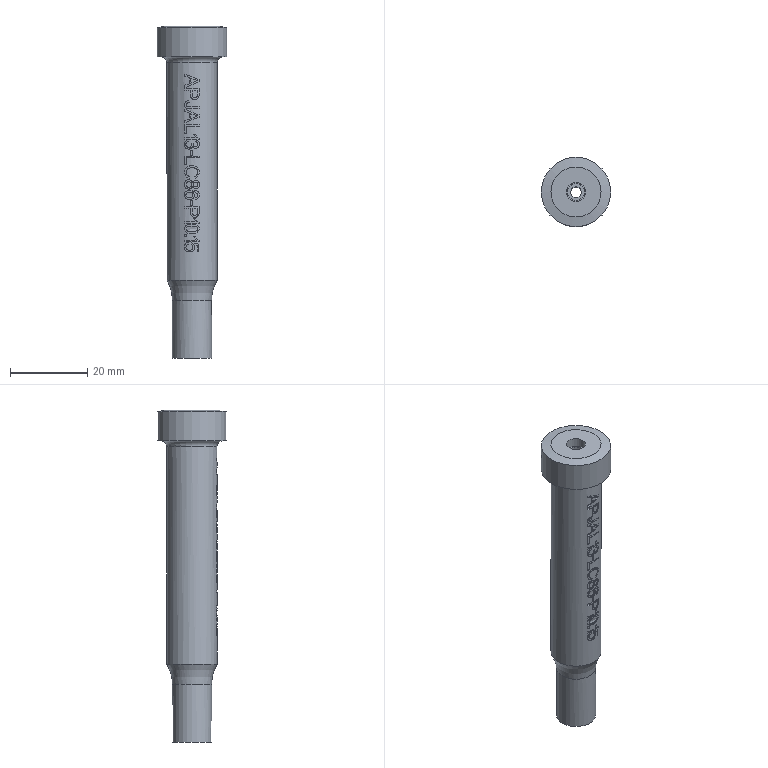Part | NX | features MI_APJAL_0254 2 | 1 solid | 218 faces | box 18 x 18 x 86 mm | volume 10368 mm3 | plane 128 | cylinder 87 | torus 2 | cone 1 | commonest cylinder face diameters 12.8 x19 13 x9 4.648 x3 5.218 x3 1.208 x2 1.331 x2